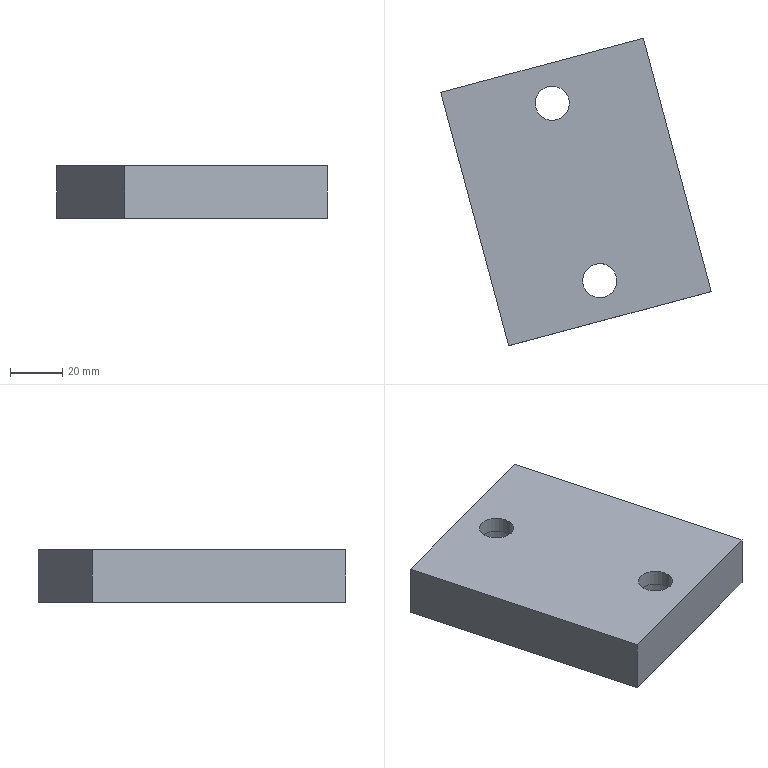Part | NX | features solid 2 | 1 solid | 12 faces | box 103.156 x 117.298 x 20 mm | volume 149611 mm3 | plane 8 | cylinder 4 | commonest cylinder face diameters 13 x2 20 x2
STEP:
#1=CARTESIAN_POINT('',(-1012.702,-146.673,-60.));
#2=VERTEX_POINT('',#1);
#3=CARTESIAN_POINT('',(-935.428,-125.967,-60.));
#4=VERTEX_POINT('',#3);
#5=CARTESIAN_POINT('',(-1012.702,-146.673,-60.));
#6=DIRECTION('',(0.9659,0.2588,0.));
#7=VECTOR('',#6,1000.);
#8=LINE('',#5,#7);
#9=EDGE_CURVE('',#2,#4,#8,.T.);
#10=ORIENTED_EDGE('',*,*,#9,.T.);
#11=CARTESIAN_POINT('',(-909.546,-222.56,-60.));
#12=VERTEX_POINT('',#11);
#13=CARTESIAN_POINT('',(-935.428,-125.967,-60.));
#14=DIRECTION('',(0.2588,-0.9659,0.));
#15=VECTOR('',#14,1000.);
#16=LINE('',#13,#15);
#17=EDGE_CURVE('',#4,#12,#16,.T.);
#18=ORIENTED_EDGE('',*,*,#17,.T.);
#19=CARTESIAN_POINT('',(-986.82,-243.265,-60.));
#20=VERTEX_POINT('',#19);
#21=CARTESIAN_POINT('',(-909.546,-222.56,-60.));
#22=DIRECTION('',(-0.9659,-0.2588,0.));
#23=VECTOR('',#22,1000.);
#24=LINE('',#21,#23);
#25=EDGE_CURVE('',#12,#20,#24,.T.);
#26=ORIENTED_EDGE('',*,*,#25,.T.);
#27=CARTESIAN_POINT('',(-986.82,-243.265,-60.));
#28=DIRECTION('',(-0.2588,0.9659,0.));
#29=VECTOR('',#28,1000.);
#30=LINE('',#27,#29);
#31=EDGE_CURVE('',#20,#2,#30,.T.);
#32=ORIENTED_EDGE('',*,*,#31,.T.);
#33=EDGE_LOOP('',(#10,#18,#26,#32));
#34=FACE_BOUND('',#33,.T.);
#35=CARTESIAN_POINT('',(-954.654,-208.764,-60.));
#36=VERTEX_POINT('',#35);
#37=CARTESIAN_POINT('',(-952.066,-218.424,-60.));
#38=DIRECTION('',(0.,0.,-1.));
#39=DIRECTION('',(-0.2588,0.9659,0.));
#40=AXIS2_PLACEMENT_3D('',#37,#38,#39);
#41=CIRCLE('',#40,10.);
#42=EDGE_CURVE('',#36,#36,#41,.T.);
#43=ORIENTED_EDGE('',*,*,#42,.F.);
#44=EDGE_LOOP('',(#43));
#45=FACE_BOUND('',#44,.T.);
#46=CARTESIAN_POINT('',(-967.595,-160.468,-60.));
#47=VERTEX_POINT('',#46);
#48=CARTESIAN_POINT('',(-970.183,-150.809,-60.));
#49=DIRECTION('',(0.,0.,1.));
#50=DIRECTION('',(0.2588,-0.9659,0.));
#51=AXIS2_PLACEMENT_3D('',#48,#49,#50);
#52=CIRCLE('',#51,10.);
#53=EDGE_CURVE('',#47,#47,#52,.T.);
#54=ORIENTED_EDGE('',*,*,#53,.T.);
#55=EDGE_LOOP('',(#54));
#56=FACE_BOUND('',#55,.T.);
#57=CARTESIAN_POINT('',(-1012.702,-146.673,-60.));
#58=DIRECTION('',(0.,0.,-1.));
#59=DIRECTION('',(0.2588,-0.9659,0.));
#60=AXIS2_PLACEMENT_3D('',#57,#58,#59);
#61=PLANE('',#60);
#62=ADVANCED_FACE('',(#34,#45,#56),#61,.T.);
#63=CARTESIAN_POINT('',(-968.501,-157.087,-40.));
#64=VERTEX_POINT('',#63);
#65=CARTESIAN_POINT('',(-970.183,-150.809,-40.));
#66=DIRECTION('',(0.,0.,1.));
#67=DIRECTION('',(0.2588,-0.9659,0.));
#68=AXIS2_PLACEMENT_3D('',#65,#66,#67);
#69=CIRCLE('',#68,6.5);
#70=EDGE_CURVE('',#64,#64,#69,.T.);
#71=ORIENTED_EDGE('',*,*,#70,.T.);
#72=EDGE_LOOP('',(#71));
#73=FACE_BOUND('',#72,.T.);
#74=CARTESIAN_POINT('',(-968.501,-157.087,-46.));
#75=VERTEX_POINT('',#74);
#76=CARTESIAN_POINT('',(-970.183,-150.809,-46.));
#77=DIRECTION('',(0.,0.,1.));
#78=DIRECTION('',(0.2588,-0.9659,0.));
#79=AXIS2_PLACEMENT_3D('',#76,#77,#78);
#80=CIRCLE('',#79,6.5);
#81=EDGE_CURVE('',#75,#75,#80,.T.);
#82=ORIENTED_EDGE('',*,*,#81,.F.);
#83=EDGE_LOOP('',(#82));
#84=FACE_BOUND('',#83,.T.);
#85=CARTESIAN_POINT('',(-970.183,-150.809,-60.));
#86=DIRECTION('',(0.,0.,1.));
#87=DIRECTION('',(-0.2588,0.9659,0.));
#88=AXIS2_PLACEMENT_3D('',#85,#86,#87);
#89=CYLINDRICAL_SURFACE('',#88,6.5);
#90=ADVANCED_FACE('',(#73,#84),#89,.F.);
#91=CARTESIAN_POINT('',(-1012.702,-146.673,-40.));
#92=VERTEX_POINT('',#91);
#93=CARTESIAN_POINT('',(-935.428,-125.967,-40.));
#94=VERTEX_POINT('',#93);
#95=CARTESIAN_POINT('',(-1012.702,-146.673,-40.));
#96=DIRECTION('',(0.9659,0.2588,0.));
#97=VECTOR('',#96,1000.);
#98=LINE('',#95,#97);
#99=EDGE_CURVE('',#92,#94,#98,.T.);
#100=ORIENTED_EDGE('',*,*,#99,.F.);
#101=CARTESIAN_POINT('',(-986.82,-243.265,-40.));
#102=VERTEX_POINT('',#101);
#103=CARTESIAN_POINT('',(-986.82,-243.265,-40.));
#104=DIRECTION('',(-0.2588,0.9659,0.));
#105=VECTOR('',#104,1000.);
#106=LINE('',#103,#105);
#107=EDGE_CURVE('',#102,#92,#106,.T.);
#108=ORIENTED_EDGE('',*,*,#107,.F.);
#109=CARTESIAN_POINT('',(-909.546,-222.56,-40.));
#110=VERTEX_POINT('',#109);
#111=CARTESIAN_POINT('',(-909.546,-222.56,-40.));
#112=DIRECTION('',(-0.9659,-0.2588,0.));
#113=VECTOR('',#112,1000.);
#114=LINE('',#111,#113);
#115=EDGE_CURVE('',#110,#102,#114,.T.);
#116=ORIENTED_EDGE('',*,*,#115,.F.);
#117=CARTESIAN_POINT('',(-935.428,-125.967,-40.));
#118=DIRECTION('',(0.2588,-0.9659,0.));
#119=VECTOR('',#118,1000.);
#120=LINE('',#117,#119);
#121=EDGE_CURVE('',#94,#110,#120,.T.);
#122=ORIENTED_EDGE('',*,*,#121,.F.);
#123=EDGE_LOOP('',(#100,#108,#116,#122));
#124=FACE_BOUND('',#123,.T.);
#125=CARTESIAN_POINT('',(-953.748,-212.145,-40.));
#126=VERTEX_POINT('',#125);
#127=CARTESIAN_POINT('',(-952.066,-218.424,-40.));
#128=DIRECTION('',(0.,0.,-1.));
#129=DIRECTION('',(-0.2588,0.9659,0.));
#130=AXIS2_PLACEMENT_3D('',#127,#128,#129);
#131=CIRCLE('',#130,6.5);
#132=EDGE_CURVE('',#126,#126,#131,.T.);
#133=ORIENTED_EDGE('',*,*,#132,.T.);
#134=EDGE_LOOP('',(#133));
#135=FACE_BOUND('',#134,.T.);
#136=ORIENTED_EDGE('',*,*,#70,.F.);
#137=EDGE_LOOP('',(#136));
#138=FACE_BOUND('',#137,.T.);
#139=CARTESIAN_POINT('',(-1012.702,-146.673,-40.));
#140=DIRECTION('',(0.,0.,-1.));
#141=DIRECTION('',(0.2588,-0.9659,0.));
#142=AXIS2_PLACEMENT_3D('',#139,#140,#141);
#143=PLANE('',#142);
#144=ADVANCED_FACE('',(#124,#135,#138),#143,.F.);
#145=ORIENTED_EDGE('',*,*,#99,.T.);
#146=CARTESIAN_POINT('',(-935.428,-125.967,-60.));
#147=DIRECTION('',(0.,0.,1.));
#148=VECTOR('',#147,1000.);
#149=LINE('',#146,#148);
#150=EDGE_CURVE('',#4,#94,#149,.T.);
#151=ORIENTED_EDGE('',*,*,#150,.F.);
#152=ORIENTED_EDGE('',*,*,#9,.F.);
#153=CARTESIAN_POINT('',(-1012.702,-146.673,-60.));
#154=DIRECTION('',(0.,0.,1.));
#155=VECTOR('',#154,1000.);
#156=LINE('',#153,#155);
#157=EDGE_CURVE('',#2,#92,#156,.T.);
#158=ORIENTED_EDGE('',*,*,#157,.T.);
#159=EDGE_LOOP('',(#145,#151,#152,#158));
#160=FACE_BOUND('',#159,.T.);
#161=CARTESIAN_POINT('',(-1012.702,-146.673,-60.));
#162=DIRECTION('',(-0.2588,0.9659,0.));
#163=DIRECTION('',(-0.9659,-0.2588,0.));
#164=AXIS2_PLACEMENT_3D('',#161,#162,#163);
#165=PLANE('',#164);
#166=ADVANCED_FACE('',(#160),#165,.T.);
#167=ORIENTED_EDGE('',*,*,#121,.T.);
#168=CARTESIAN_POINT('',(-909.546,-222.56,-60.));
#169=DIRECTION('',(0.,0.,1.));
#170=VECTOR('',#169,1000.);
#171=LINE('',#168,#170);
#172=EDGE_CURVE('',#12,#110,#171,.T.);
#173=ORIENTED_EDGE('',*,*,#172,.F.);
#174=ORIENTED_EDGE('',*,*,#17,.F.);
#175=ORIENTED_EDGE('',*,*,#150,.T.);
#176=EDGE_LOOP('',(#167,#173,#174,#175));
#177=FACE_BOUND('',#176,.T.);
#178=CARTESIAN_POINT('',(-935.428,-125.967,-60.));
#179=DIRECTION('',(0.9659,0.2588,0.));
#180=DIRECTION('',(0.,0.,-1.));
#181=AXIS2_PLACEMENT_3D('',#178,#179,#180);
#182=PLANE('',#181);
#183=ADVANCED_FACE('',(#177),#182,.T.);
#184=ORIENTED_EDGE('',*,*,#115,.T.);
#185=CARTESIAN_POINT('',(-986.82,-243.265,-60.));
#186=DIRECTION('',(0.,0.,1.));
#187=VECTOR('',#186,1000.);
#188=LINE('',#185,#187);
#189=EDGE_CURVE('',#20,#102,#188,.T.);
#190=ORIENTED_EDGE('',*,*,#189,.F.);
#191=ORIENTED_EDGE('',*,*,#25,.F.);
#192=ORIENTED_EDGE('',*,*,#172,.T.);
#193=EDGE_LOOP('',(#184,#190,#191,#192));
#194=FACE_BOUND('',#193,.T.);
#195=CARTESIAN_POINT('',(-909.546,-222.56,-60.));
#196=DIRECTION('',(0.2588,-0.9659,0.));
#197=DIRECTION('',(0.9659,0.2588,0.));
#198=AXIS2_PLACEMENT_3D('',#195,#196,#197);
#199=PLANE('',#198);
#200=ADVANCED_FACE('',(#194),#199,.T.);
#201=ORIENTED_EDGE('',*,*,#107,.T.);
#202=ORIENTED_EDGE('',*,*,#157,.F.);
#203=ORIENTED_EDGE('',*,*,#31,.F.);
#204=ORIENTED_EDGE('',*,*,#189,.T.);
#205=EDGE_LOOP('',(#201,#202,#203,#204));
#206=FACE_BOUND('',#205,.T.);
#207=CARTESIAN_POINT('',(-986.82,-243.265,-60.));
#208=DIRECTION('',(-0.9659,-0.2588,0.));
#209=DIRECTION('',(0.2588,-0.9659,0.));
#210=AXIS2_PLACEMENT_3D('',#207,#208,#209);
#211=PLANE('',#210);
#212=ADVANCED_FACE('',(#206),#211,.T.);
#213=CARTESIAN_POINT('',(-953.748,-212.145,-46.));
#214=VERTEX_POINT('',#213);
#215=CARTESIAN_POINT('',(-952.066,-218.424,-46.));
#216=DIRECTION('',(0.,0.,-1.));
#217=DIRECTION('',(-0.2588,0.9659,0.));
#218=AXIS2_PLACEMENT_3D('',#215,#216,#217);
#219=CIRCLE('',#218,6.5);
#220=EDGE_CURVE('',#214,#214,#219,.F.);
#221=ORIENTED_EDGE('',*,*,#220,.F.);
#222=EDGE_LOOP('',(#221));
#223=FACE_BOUND('',#222,.T.);
#224=ORIENTED_EDGE('',*,*,#132,.F.);
#225=EDGE_LOOP('',(#224));
#226=FACE_BOUND('',#225,.T.);
#227=CARTESIAN_POINT('',(-952.066,-218.424,-60.));
#228=DIRECTION('',(0.,0.,1.));
#229=DIRECTION('',(-0.2588,0.9659,0.));
#230=AXIS2_PLACEMENT_3D('',#227,#228,#229);
#231=CYLINDRICAL_SURFACE('',#230,6.5);
#232=ADVANCED_FACE('',(#223,#226),#231,.F.);
#233=CARTESIAN_POINT('',(-954.654,-208.764,-46.));
#234=VERTEX_POINT('',#233);
#235=CARTESIAN_POINT('',(-952.066,-218.424,-46.));
#236=DIRECTION('',(0.,0.,-1.));
#237=DIRECTION('',(-0.2588,0.9659,0.));
#238=AXIS2_PLACEMENT_3D('',#235,#236,#237);
#239=CIRCLE('',#238,10.);
#240=EDGE_CURVE('',#234,#234,#239,.T.);
#241=ORIENTED_EDGE('',*,*,#240,.T.);
#242=EDGE_LOOP('',(#241));
#243=FACE_BOUND('',#242,.T.);
#244=ORIENTED_EDGE('',*,*,#220,.T.);
#245=EDGE_LOOP('',(#244));
#246=FACE_BOUND('',#245,.T.);
#247=CARTESIAN_POINT('',(-952.066,-218.424,-46.));
#248=DIRECTION('',(0.,0.,1.));
#249=DIRECTION('',(-0.2588,0.9659,0.));
#250=AXIS2_PLACEMENT_3D('',#247,#248,#249);
#251=PLANE('',#250);
#252=ADVANCED_FACE('',(#243,#246),#251,.F.);
#253=ORIENTED_EDGE('',*,*,#42,.T.);
#254=EDGE_LOOP('',(#253));
#255=FACE_BOUND('',#254,.T.);
#256=ORIENTED_EDGE('',*,*,#240,.F.);
#257=EDGE_LOOP('',(#256));
#258=FACE_BOUND('',#257,.T.);
#259=CARTESIAN_POINT('',(-952.066,-218.424,-60.));
#260=DIRECTION('',(0.,0.,1.));
#261=DIRECTION('',(-0.2588,0.9659,0.));
#262=AXIS2_PLACEMENT_3D('',#259,#260,#261);
#263=CYLINDRICAL_SURFACE('',#262,10.);
#264=ADVANCED_FACE('',(#255,#258),#263,.F.);
#265=ORIENTED_EDGE('',*,*,#53,.F.);
#266=EDGE_LOOP('',(#265));
#267=FACE_BOUND('',#266,.T.);
#268=CARTESIAN_POINT('',(-967.595,-160.468,-46.));
#269=VERTEX_POINT('',#268);
#270=CARTESIAN_POINT('',(-970.183,-150.809,-46.));
#271=DIRECTION('',(0.,0.,1.));
#272=DIRECTION('',(0.2588,-0.9659,0.));
#273=AXIS2_PLACEMENT_3D('',#270,#271,#272);
#274=CIRCLE('',#273,10.);
#275=EDGE_CURVE('',#269,#269,#274,.T.);
#276=ORIENTED_EDGE('',*,*,#275,.T.);
#277=EDGE_LOOP('',(#276));
#278=FACE_BOUND('',#277,.T.);
#279=CARTESIAN_POINT('',(-970.183,-150.809,-60.));
#280=DIRECTION('',(0.,0.,1.));
#281=DIRECTION('',(-0.2588,0.9659,0.));
#282=AXIS2_PLACEMENT_3D('',#279,#280,#281);
#283=CYLINDRICAL_SURFACE('',#282,10.);
#284=ADVANCED_FACE('',(#267,#278),#283,.F.);
#285=ORIENTED_EDGE('',*,*,#81,.T.);
#286=EDGE_LOOP('',(#285));
#287=FACE_BOUND('',#286,.T.);
#288=ORIENTED_EDGE('',*,*,#275,.F.);
#289=EDGE_LOOP('',(#288));
#290=FACE_BOUND('',#289,.T.);
#291=CARTESIAN_POINT('',(-970.183,-150.809,-46.));
#292=DIRECTION('',(0.,0.,-1.));
#293=DIRECTION('',(0.2588,-0.9659,0.));
#294=AXIS2_PLACEMENT_3D('',#291,#292,#293);
#295=PLANE('',#294);
#296=ADVANCED_FACE('',(#287,#290),#295,.T.);
#297=CLOSED_SHELL('',(#62,#90,#144,#166,#183,#200,#212,#232,#252,#264,#284,#296));
#298=MANIFOLD_SOLID_BREP('',#297);
#299=(LENGTH_UNIT()NAMED_UNIT(*)SI_UNIT(.MILLI.,.METRE.));
#300=UNCERTAINTY_MEASURE_WITH_UNIT(LENGTH_MEASURE(0.00001),#299,'','');
#301=(NAMED_UNIT(*)PLANE_ANGLE_UNIT()SI_UNIT($,.RADIAN.));
#302=(NAMED_UNIT(*)SI_UNIT($,.STERADIAN.)SOLID_ANGLE_UNIT());
#303=(GEOMETRIC_REPRESENTATION_CONTEXT(3)GLOBAL_UNCERTAINTY_ASSIGNED_CONTEXT((#300))GLOBAL_UNIT_ASSIGNED_CONTEXT((#299,#301,#302))REPRESENTATION_CONTEXT('',''));
#304=ADVANCED_BREP_SHAPE_REPRESENTATION('',(#298),#303);